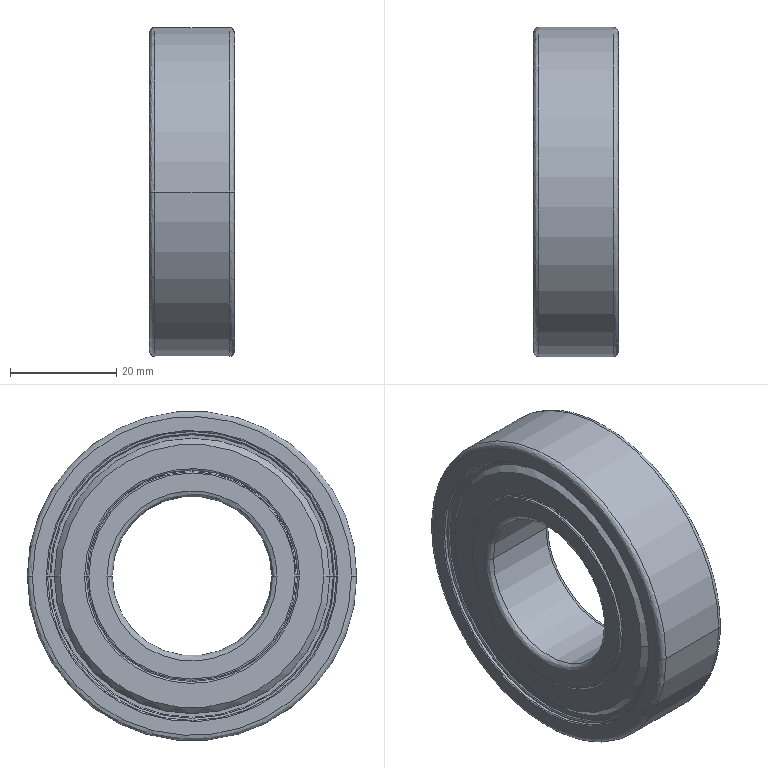Part | SolidWorks | features BaseBody 1 | 1 solid | 132 faces | box 16 x 62 x 62 mm | volume 30543 mm3 | spline 52 | cone 40 | cylinder 28 | plane 12 | commonest cylinder face diameters 39.2 x4 39.8 x4 40.4 x4 40.8 x4 52.2 x4 54.4 x4